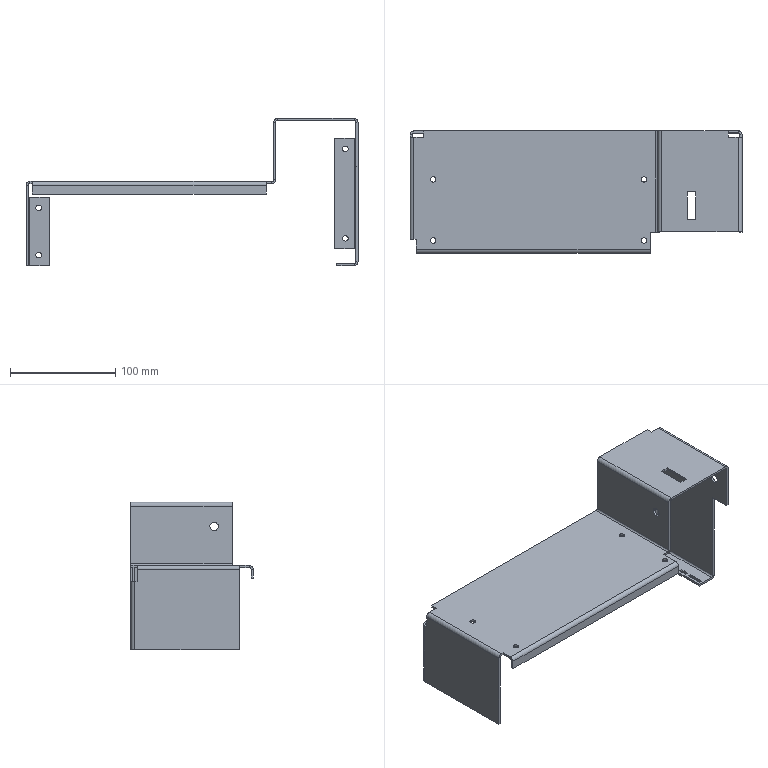Part | STEP file | 8XS043017.1~5 | 1 solid | 114 faces | box 315 x 116 x 140 mm | volume 129914 mm3 | plane 78 | cylinder 36 | commonest cylinder face diameters 5.2 x16 3.2 x8 7.2 x8 8 x4